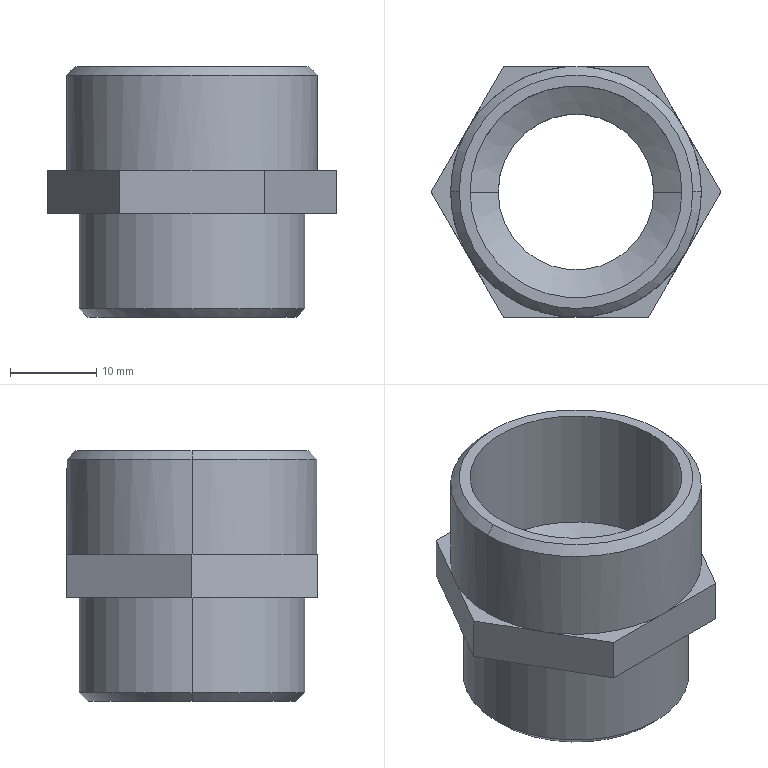Part | SolidWorks | features ICE 3, Chamfer 1, Extrusion 1, HoleWzd 1 | 1 solid | 29 faces | box 33.486 x 29 x 29 mm | volume 7069 mm3 | plane 15 | cylinder 8 | cone 6 | commonest cylinder face diameters 18 x2 24.5 x2 26.1 x2 29 x2
STEP:
#1=CARTESIAN_POINT('',(13.5,0.,14.5));
#2=VERTEX_POINT('',#1);
#3=CARTESIAN_POINT('',(-13.5,0.,14.5));
#4=VERTEX_POINT('',#3);
#5=CARTESIAN_POINT('',(0.,0.,14.5));
#6=DIRECTION('',(0.,0.,1.));
#7=DIRECTION('',(1.,0.,0.));
#8=AXIS2_PLACEMENT_3D('',#5,#6,#7);
#9=CIRCLE('',#8,13.5);
#10=EDGE_CURVE('',#2,#4,#9,.T.);
#11=ORIENTED_EDGE('',*,*,#10,.F.);
#12=CARTESIAN_POINT('',(14.5,0.,13.5));
#13=VERTEX_POINT('',#12);
#14=CARTESIAN_POINT('',(13.5,0.,14.5));
#15=DIRECTION('',(0.7071,0.,-0.7071));
#16=VECTOR('',#15,1000.);
#17=LINE('',#14,#16);
#18=EDGE_CURVE('',#2,#13,#17,.T.);
#19=ORIENTED_EDGE('',*,*,#18,.T.);
#20=CARTESIAN_POINT('',(-14.5,0.,13.5));
#21=VERTEX_POINT('',#20);
#22=CARTESIAN_POINT('',(0.,0.,13.5));
#23=DIRECTION('',(0.,0.,-1.));
#24=DIRECTION('',(1.,0.,0.));
#25=AXIS2_PLACEMENT_3D('',#22,#23,#24);
#26=CIRCLE('',#25,14.5);
#27=EDGE_CURVE('',#21,#13,#26,.T.);
#28=ORIENTED_EDGE('',*,*,#27,.F.);
#29=CARTESIAN_POINT('',(-13.5,0.,14.5));
#30=DIRECTION('',(-0.7071,0.,-0.7071));
#31=VECTOR('',#30,1000.);
#32=LINE('',#29,#31);
#33=EDGE_CURVE('',#4,#21,#32,.T.);
#34=ORIENTED_EDGE('',*,*,#33,.F.);
#35=EDGE_LOOP('',(#11,#19,#28,#34));
#36=FACE_OUTER_BOUND('',#35,.T.);
#37=CARTESIAN_POINT('',(0.,0.,14.5));
#38=DIRECTION('',(0.,0.,-1.));
#39=DIRECTION('',(-1.,0.,0.));
#40=AXIS2_PLACEMENT_3D('',#37,#38,#39);
#41=CONICAL_SURFACE('',#40,13.5,0.7854);
#42=ADVANCED_FACE('',(#36),#41,.T.);
#43=CARTESIAN_POINT('',(-12.05,0.,-14.5));
#44=VERTEX_POINT('',#43);
#45=CARTESIAN_POINT('',(12.05,0.,-14.5));
#46=VERTEX_POINT('',#45);
#47=CARTESIAN_POINT('',(0.,0.,-14.5));
#48=DIRECTION('',(0.,0.,-1.));
#49=DIRECTION('',(-1.,0.,0.));
#50=AXIS2_PLACEMENT_3D('',#47,#48,#49);
#51=CIRCLE('',#50,12.05);
#52=EDGE_CURVE('',#44,#46,#51,.T.);
#53=ORIENTED_EDGE('',*,*,#52,.F.);
#54=CARTESIAN_POINT('',(-13.05,0.,-13.5));
#55=VERTEX_POINT('',#54);
#56=CARTESIAN_POINT('',(-12.05,0.,-14.5));
#57=DIRECTION('',(-0.7071,0.,0.7071));
#58=VECTOR('',#57,1000.);
#59=LINE('',#56,#58);
#60=EDGE_CURVE('',#44,#55,#59,.T.);
#61=ORIENTED_EDGE('',*,*,#60,.T.);
#62=CARTESIAN_POINT('',(13.05,0.,-13.5));
#63=VERTEX_POINT('',#62);
#64=CARTESIAN_POINT('',(0.,0.,-13.5));
#65=DIRECTION('',(0.,0.,1.));
#66=DIRECTION('',(-1.,0.,0.));
#67=AXIS2_PLACEMENT_3D('',#64,#65,#66);
#68=CIRCLE('',#67,13.05);
#69=EDGE_CURVE('',#63,#55,#68,.T.);
#70=ORIENTED_EDGE('',*,*,#69,.F.);
#71=CARTESIAN_POINT('',(12.05,0.,-14.5));
#72=DIRECTION('',(0.7071,0.,0.7071));
#73=VECTOR('',#72,1000.);
#74=LINE('',#71,#73);
#75=EDGE_CURVE('',#46,#63,#74,.T.);
#76=ORIENTED_EDGE('',*,*,#75,.F.);
#77=EDGE_LOOP('',(#53,#61,#70,#76));
#78=FACE_OUTER_BOUND('',#77,.T.);
#79=CARTESIAN_POINT('',(0.,0.,-14.5));
#80=DIRECTION('',(0.,0.,1.));
#81=DIRECTION('',(1.,0.,0.));
#82=AXIS2_PLACEMENT_3D('',#79,#80,#81);
#83=CONICAL_SURFACE('',#82,12.05,0.7854);
#84=ADVANCED_FACE('',(#78),#83,.T.);
#85=CARTESIAN_POINT('',(-12.25,0.,-0.5));
#86=VERTEX_POINT('',#85);
#87=CARTESIAN_POINT('',(12.25,0.,-0.5));
#88=VERTEX_POINT('',#87);
#89=CARTESIAN_POINT('',(0.,0.,-0.5));
#90=DIRECTION('',(0.,0.,1.));
#91=DIRECTION('',(1.,0.,0.));
#92=AXIS2_PLACEMENT_3D('',#89,#90,#91);
#93=CIRCLE('',#92,12.25);
#94=EDGE_CURVE('',#86,#88,#93,.T.);
#95=ORIENTED_EDGE('',*,*,#94,.F.);
#96=CARTESIAN_POINT('',(-12.25,0.,14.5));
#97=VERTEX_POINT('',#96);
#98=CARTESIAN_POINT('',(-12.25,0.,14.5));
#99=DIRECTION('',(0.,0.,1.));
#100=VECTOR('',#99,1000.);
#101=LINE('',#98,#100);
#102=EDGE_CURVE('',#86,#97,#101,.T.);
#103=ORIENTED_EDGE('',*,*,#102,.T.);
#104=CARTESIAN_POINT('',(12.25,0.,14.5));
#105=VERTEX_POINT('',#104);
#106=CARTESIAN_POINT('',(0.,0.,14.5));
#107=DIRECTION('',(0.,0.,1.));
#108=DIRECTION('',(1.,0.,0.));
#109=AXIS2_PLACEMENT_3D('',#106,#107,#108);
#110=CIRCLE('',#109,12.25);
#111=EDGE_CURVE('',#97,#105,#110,.T.);
#112=ORIENTED_EDGE('',*,*,#111,.T.);
#113=CARTESIAN_POINT('',(12.25,0.,14.5));
#114=DIRECTION('',(0.,0.,1.));
#115=VECTOR('',#114,1000.);
#116=LINE('',#113,#115);
#117=EDGE_CURVE('',#88,#105,#116,.T.);
#118=ORIENTED_EDGE('',*,*,#117,.F.);
#119=EDGE_LOOP('',(#95,#103,#112,#118));
#120=FACE_OUTER_BOUND('',#119,.T.);
#121=CARTESIAN_POINT('',(0.,0.,14.5));
#122=DIRECTION('',(0.,0.,1.));
#123=DIRECTION('',(1.,0.,0.));
#124=AXIS2_PLACEMENT_3D('',#121,#122,#123);
#125=CYLINDRICAL_SURFACE('',#124,12.25);
#126=ADVANCED_FACE('',(#120),#125,.F.);
#127=CARTESIAN_POINT('',(-9.,0.,-2.453));
#128=VERTEX_POINT('',#127);
#129=CARTESIAN_POINT('',(9.,0.,-2.453));
#130=VERTEX_POINT('',#129);
#131=CARTESIAN_POINT('',(0.,0.,-2.453));
#132=DIRECTION('',(0.,0.,1.));
#133=DIRECTION('',(1.,0.,0.));
#134=AXIS2_PLACEMENT_3D('',#131,#132,#133);
#135=CIRCLE('',#134,9.);
#136=EDGE_CURVE('',#128,#130,#135,.T.);
#137=ORIENTED_EDGE('',*,*,#136,.F.);
#138=CARTESIAN_POINT('',(-12.25,0.,-0.5));
#139=DIRECTION('',(-0.8572,0.,0.515));
#140=VECTOR('',#139,1000.);
#141=LINE('',#138,#140);
#142=EDGE_CURVE('',#128,#86,#141,.T.);
#143=ORIENTED_EDGE('',*,*,#142,.T.);
#144=ORIENTED_EDGE('',*,*,#94,.T.);
#145=CARTESIAN_POINT('',(12.25,0.,-0.5));
#146=DIRECTION('',(0.8572,0.,0.515));
#147=VECTOR('',#146,1000.);
#148=LINE('',#145,#147);
#149=EDGE_CURVE('',#130,#88,#148,.T.);
#150=ORIENTED_EDGE('',*,*,#149,.F.);
#151=EDGE_LOOP('',(#137,#143,#144,#150));
#152=FACE_OUTER_BOUND('',#151,.T.);
#153=CARTESIAN_POINT('',(0.,0.,-0.5));
#154=DIRECTION('',(0.,0.,1.));
#155=DIRECTION('',(1.,0.,0.));
#156=AXIS2_PLACEMENT_3D('',#153,#154,#155);
#157=CONICAL_SURFACE('',#156,12.25,1.03);
#158=ADVANCED_FACE('',(#152),#157,.F.);
#159=ORIENTED_EDGE('',*,*,#27,.T.);
#160=CARTESIAN_POINT('',(14.5,0.,2.5));
#161=VERTEX_POINT('',#160);
#162=CARTESIAN_POINT('',(14.5,0.,14.5));
#163=DIRECTION('',(0.,0.,-1.));
#164=VECTOR('',#163,1000.);
#165=LINE('',#162,#164);
#166=EDGE_CURVE('',#13,#161,#165,.T.);
#167=ORIENTED_EDGE('',*,*,#166,.T.);
#168=CARTESIAN_POINT('',(12.557,7.25,2.5));
#169=VERTEX_POINT('',#168);
#170=CARTESIAN_POINT('',(0.,0.,2.5));
#171=DIRECTION('',(0.,0.,1.));
#172=DIRECTION('',(1.,0.,0.));
#173=AXIS2_PLACEMENT_3D('',#170,#171,#172);
#174=CIRCLE('',#173,14.5);
#175=EDGE_CURVE('',#161,#169,#174,.T.);
#176=ORIENTED_EDGE('',*,*,#175,.T.);
#177=CARTESIAN_POINT('',(0.,14.5,2.5));
#178=VERTEX_POINT('',#177);
#179=CARTESIAN_POINT('',(0.,0.,2.5));
#180=DIRECTION('',(0.,0.,1.));
#181=DIRECTION('',(1.,0.,0.));
#182=AXIS2_PLACEMENT_3D('',#179,#180,#181);
#183=CIRCLE('',#182,14.5);
#184=EDGE_CURVE('',#169,#178,#183,.T.);
#185=ORIENTED_EDGE('',*,*,#184,.T.);
#186=CARTESIAN_POINT('',(-12.557,7.25,2.5));
#187=VERTEX_POINT('',#186);
#188=CARTESIAN_POINT('',(0.,0.,2.5));
#189=DIRECTION('',(0.,0.,1.));
#190=DIRECTION('',(1.,0.,0.));
#191=AXIS2_PLACEMENT_3D('',#188,#189,#190);
#192=CIRCLE('',#191,14.5);
#193=EDGE_CURVE('',#178,#187,#192,.T.);
#194=ORIENTED_EDGE('',*,*,#193,.T.);
#195=CARTESIAN_POINT('',(-14.5,0.,2.5));
#196=VERTEX_POINT('',#195);
#197=CARTESIAN_POINT('',(0.,0.,2.5));
#198=DIRECTION('',(0.,0.,1.));
#199=DIRECTION('',(1.,0.,0.));
#200=AXIS2_PLACEMENT_3D('',#197,#198,#199);
#201=CIRCLE('',#200,14.5);
#202=EDGE_CURVE('',#187,#196,#201,.T.);
#203=ORIENTED_EDGE('',*,*,#202,.T.);
#204=CARTESIAN_POINT('',(-14.5,0.,14.5));
#205=DIRECTION('',(0.,0.,-1.));
#206=VECTOR('',#205,1000.);
#207=LINE('',#204,#206);
#208=EDGE_CURVE('',#21,#196,#207,.T.);
#209=ORIENTED_EDGE('',*,*,#208,.F.);
#210=EDGE_LOOP('',(#159,#167,#176,#185,#194,#203,#209));
#211=FACE_OUTER_BOUND('',#210,.T.);
#212=CARTESIAN_POINT('',(0.,0.,14.5));
#213=DIRECTION('',(0.,0.,-1.));
#214=DIRECTION('',(-1.,0.,0.));
#215=AXIS2_PLACEMENT_3D('',#212,#213,#214);
#216=CYLINDRICAL_SURFACE('',#215,14.5);
#217=ADVANCED_FACE('',(#211),#216,.T.);
#218=ORIENTED_EDGE('',*,*,#136,.T.);
#219=CARTESIAN_POINT('',(9.,0.,-14.5));
#220=VERTEX_POINT('',#219);
#221=CARTESIAN_POINT('',(9.,0.,2.501));
#222=DIRECTION('',(0.,0.,-1.));
#223=VECTOR('',#222,1000.);
#224=LINE('',#221,#223);
#225=EDGE_CURVE('',#130,#220,#224,.T.);
#226=ORIENTED_EDGE('',*,*,#225,.T.);
#227=CARTESIAN_POINT('',(-9.,0.,-14.5));
#228=VERTEX_POINT('',#227);
#229=CARTESIAN_POINT('',(0.,0.,-14.5));
#230=DIRECTION('',(0.,0.,-1.));
#231=DIRECTION('',(-1.,0.,0.));
#232=AXIS2_PLACEMENT_3D('',#229,#230,#231);
#233=CIRCLE('',#232,9.);
#234=EDGE_CURVE('',#220,#228,#233,.T.);
#235=ORIENTED_EDGE('',*,*,#234,.T.);
#236=CARTESIAN_POINT('',(-9.,0.,2.501));
#237=DIRECTION('',(0.,0.,-1.));
#238=VECTOR('',#237,1000.);
#239=LINE('',#236,#238);
#240=EDGE_CURVE('',#128,#228,#239,.T.);
#241=ORIENTED_EDGE('',*,*,#240,.F.);
#242=EDGE_LOOP('',(#218,#226,#235,#241));
#243=FACE_OUTER_BOUND('',#242,.T.);
#244=CARTESIAN_POINT('',(0.,0.,2.501));
#245=DIRECTION('',(0.,0.,-1.));
#246=DIRECTION('',(-1.,0.,0.));
#247=AXIS2_PLACEMENT_3D('',#244,#245,#246);
#248=CYLINDRICAL_SURFACE('',#247,9.);
#249=ADVANCED_FACE('',(#243),#248,.F.);
#250=ORIENTED_EDGE('',*,*,#69,.T.);
#251=CARTESIAN_POINT('',(-13.05,0.,-2.5));
#252=VERTEX_POINT('',#251);
#253=CARTESIAN_POINT('',(-13.05,0.,-14.5));
#254=DIRECTION('',(0.,0.,1.));
#255=VECTOR('',#254,1000.);
#256=LINE('',#253,#255);
#257=EDGE_CURVE('',#55,#252,#256,.T.);
#258=ORIENTED_EDGE('',*,*,#257,.T.);
#259=CARTESIAN_POINT('',(13.05,0.,-2.5));
#260=VERTEX_POINT('',#259);
#261=CARTESIAN_POINT('',(0.,0.,-2.5));
#262=DIRECTION('',(0.,0.,-1.));
#263=DIRECTION('',(-1.,0.,0.));
#264=AXIS2_PLACEMENT_3D('',#261,#262,#263);
#265=CIRCLE('',#264,13.05);
#266=EDGE_CURVE('',#252,#260,#265,.T.);
#267=ORIENTED_EDGE('',*,*,#266,.T.);
#268=CARTESIAN_POINT('',(13.05,0.,-14.5));
#269=DIRECTION('',(0.,0.,1.));
#270=VECTOR('',#269,1000.);
#271=LINE('',#268,#270);
#272=EDGE_CURVE('',#63,#260,#271,.T.);
#273=ORIENTED_EDGE('',*,*,#272,.F.);
#274=EDGE_LOOP('',(#250,#258,#267,#273));
#275=FACE_OUTER_BOUND('',#274,.T.);
#276=CARTESIAN_POINT('',(0.,0.,-14.5));
#277=DIRECTION('',(0.,0.,1.));
#278=DIRECTION('',(1.,0.,0.));
#279=AXIS2_PLACEMENT_3D('',#276,#277,#278);
#280=CYLINDRICAL_SURFACE('',#279,13.05);
#281=ADVANCED_FACE('',(#275),#280,.T.);
#282=ORIENTED_EDGE('',*,*,#184,.F.);
#283=CARTESIAN_POINT('',(8.372,14.5,2.5));
#284=VERTEX_POINT('',#283);
#285=CARTESIAN_POINT('',(16.743,0.,2.5));
#286=DIRECTION('',(-0.5,0.866,0.));
#287=VECTOR('',#286,1000.);
#288=LINE('',#285,#287);
#289=EDGE_CURVE('',#169,#284,#288,.T.);
#290=ORIENTED_EDGE('',*,*,#289,.T.);
#291=CARTESIAN_POINT('',(8.372,14.5,2.5));
#292=DIRECTION('',(-1.,0.,0.));
#293=VECTOR('',#292,1000.);
#294=LINE('',#291,#293);
#295=EDGE_CURVE('',#284,#178,#294,.T.);
#296=ORIENTED_EDGE('',*,*,#295,.T.);
#297=EDGE_LOOP('',(#282,#290,#296));
#298=FACE_OUTER_BOUND('',#297,.T.);
#299=CARTESIAN_POINT('',(0.,0.,2.5));
#300=DIRECTION('',(0.,0.,1.));
#301=DIRECTION('',(1.,0.,0.));
#302=AXIS2_PLACEMENT_3D('',#299,#300,#301);
#303=PLANE('',#302);
#304=ADVANCED_FACE('',(#298),#303,.T.);
#305=ORIENTED_EDGE('',*,*,#193,.F.);
#306=CARTESIAN_POINT('',(-8.372,14.5,2.5));
#307=VERTEX_POINT('',#306);
#308=CARTESIAN_POINT('',(8.372,14.5,2.5));
#309=DIRECTION('',(-1.,0.,0.));
#310=VECTOR('',#309,1000.);
#311=LINE('',#308,#310);
#312=EDGE_CURVE('',#178,#307,#311,.T.);
#313=ORIENTED_EDGE('',*,*,#312,.T.);
#314=CARTESIAN_POINT('',(-8.372,14.5,2.5));
#315=DIRECTION('',(-0.5,-0.866,0.));
#316=VECTOR('',#315,1000.);
#317=LINE('',#314,#316);
#318=EDGE_CURVE('',#307,#187,#317,.T.);
#319=ORIENTED_EDGE('',*,*,#318,.T.);
#320=EDGE_LOOP('',(#305,#313,#319));
#321=FACE_OUTER_BOUND('',#320,.T.);
#322=CARTESIAN_POINT('',(0.,0.,2.5));
#323=DIRECTION('',(0.,0.,1.));
#324=DIRECTION('',(1.,0.,0.));
#325=AXIS2_PLACEMENT_3D('',#322,#323,#324);
#326=PLANE('',#325);
#327=ADVANCED_FACE('',(#321),#326,.T.);
#328=ORIENTED_EDGE('',*,*,#202,.F.);
#329=CARTESIAN_POINT('',(-16.743,0.,2.5));
#330=VERTEX_POINT('',#329);
#331=CARTESIAN_POINT('',(-8.372,14.5,2.5));
#332=DIRECTION('',(-0.5,-0.866,0.));
#333=VECTOR('',#332,1000.);
#334=LINE('',#331,#333);
#335=EDGE_CURVE('',#187,#330,#334,.T.);
#336=ORIENTED_EDGE('',*,*,#335,.T.);
#337=CARTESIAN_POINT('',(-12.557,-7.25,2.5));
#338=VERTEX_POINT('',#337);
#339=CARTESIAN_POINT('',(-16.743,0.,2.5));
#340=DIRECTION('',(0.5,-0.866,0.));
#341=VECTOR('',#340,1000.);
#342=LINE('',#339,#341);
#343=EDGE_CURVE('',#330,#338,#342,.T.);
#344=ORIENTED_EDGE('',*,*,#343,.T.);
#345=CARTESIAN_POINT('',(0.,0.,2.5));
#346=DIRECTION('',(0.,0.,1.));
#347=DIRECTION('',(1.,0.,0.));
#348=AXIS2_PLACEMENT_3D('',#345,#346,#347);
#349=CIRCLE('',#348,14.5);
#350=EDGE_CURVE('',#196,#338,#349,.T.);
#351=ORIENTED_EDGE('',*,*,#350,.F.);
#352=EDGE_LOOP('',(#328,#336,#344,#351));
#353=FACE_OUTER_BOUND('',#352,.T.);
#354=CARTESIAN_POINT('',(0.,0.,2.5));
#355=DIRECTION('',(0.,0.,1.));
#356=DIRECTION('',(1.,0.,0.));
#357=AXIS2_PLACEMENT_3D('',#354,#355,#356);
#358=PLANE('',#357);
#359=ADVANCED_FACE('',(#353),#358,.T.);
#360=CARTESIAN_POINT('',(0.,-14.5,2.5));
#361=VERTEX_POINT('',#360);
#362=CARTESIAN_POINT('',(0.,0.,2.5));
#363=DIRECTION('',(0.,0.,1.));
#364=DIRECTION('',(1.,0.,0.));
#365=AXIS2_PLACEMENT_3D('',#362,#363,#364);
#366=CIRCLE('',#365,14.5);
#367=EDGE_CURVE('',#338,#361,#366,.T.);
#368=ORIENTED_EDGE('',*,*,#367,.F.);
#369=CARTESIAN_POINT('',(-8.372,-14.5,2.5));
#370=VERTEX_POINT('',#369);
#371=CARTESIAN_POINT('',(-16.743,0.,2.5));
#372=DIRECTION('',(0.5,-0.866,0.));
#373=VECTOR('',#372,1000.);
#374=LINE('',#371,#373);
#375=EDGE_CURVE('',#338,#370,#374,.T.);
#376=ORIENTED_EDGE('',*,*,#375,.T.);
#377=CARTESIAN_POINT('',(-8.372,-14.5,2.5));
#378=DIRECTION('',(1.,0.,0.));
#379=VECTOR('',#378,1000.);
#380=LINE('',#377,#379);
#381=EDGE_CURVE('',#370,#361,#380,.T.);
#382=ORIENTED_EDGE('',*,*,#381,.T.);
#383=EDGE_LOOP('',(#368,#376,#382));
#384=FACE_OUTER_BOUND('',#383,.T.);
#385=CARTESIAN_POINT('',(0.,0.,2.5));
#386=DIRECTION('',(0.,0.,1.));
#387=DIRECTION('',(1.,0.,0.));
#388=AXIS2_PLACEMENT_3D('',#385,#386,#387);
#389=PLANE('',#388);
#390=ADVANCED_FACE('',(#384),#389,.T.);
#391=CARTESIAN_POINT('',(12.557,-7.25,2.5));
#392=VERTEX_POINT('',#391);
#393=CARTESIAN_POINT('',(0.,0.,2.5));
#394=DIRECTION('',(0.,0.,1.));
#395=DIRECTION('',(1.,0.,0.));
#396=AXIS2_PLACEMENT_3D('',#393,#394,#395);
#397=CIRCLE('',#396,14.5);
#398=EDGE_CURVE('',#361,#392,#397,.T.);
#399=ORIENTED_EDGE('',*,*,#398,.F.);
#400=CARTESIAN_POINT('',(8.372,-14.5,2.5));
#401=VERTEX_POINT('',#400);
#402=CARTESIAN_POINT('',(-8.372,-14.5,2.5));
#403=DIRECTION('',(1.,0.,0.));
#404=VECTOR('',#403,1000.);
#405=LINE('',#402,#404);
#406=EDGE_CURVE('',#361,#401,#405,.T.);
#407=ORIENTED_EDGE('',*,*,#406,.T.);
#408=CARTESIAN_POINT('',(8.372,-14.5,2.5));
#409=DIRECTION('',(0.5,0.866,0.));
#410=VECTOR('',#409,1000.);
#411=LINE('',#408,#410);
#412=EDGE_CURVE('',#401,#392,#411,.T.);
#413=ORIENTED_EDGE('',*,*,#412,.T.);
#414=EDGE_LOOP('',(#399,#407,#413));
#415=FACE_OUTER_BOUND('',#414,.T.);
#416=CARTESIAN_POINT('',(0.,0.,2.5));
#417=DIRECTION('',(0.,0.,1.));
#418=DIRECTION('',(1.,0.,0.));
#419=AXIS2_PLACEMENT_3D('',#416,#417,#418);
#420=PLANE('',#419);
#421=ADVANCED_FACE('',(#415),#420,.T.);
#422=CARTESIAN_POINT('',(8.372,-14.5,-2.5));
#423=VERTEX_POINT('',#422);
#424=CARTESIAN_POINT('',(16.743,0.,-2.5));
#425=VERTEX_POINT('',#424);
#426=CARTESIAN_POINT('',(8.372,-14.5,-2.5));
#427=DIRECTION('',(0.5,0.866,0.));
#428=VECTOR('',#427,1000.);
#429=LINE('',#426,#428);
#430=EDGE_CURVE('',#423,#425,#429,.T.);
#431=ORIENTED_EDGE('',*,*,#430,.T.);
#432=CARTESIAN_POINT('',(16.743,0.,2.5));
#433=VERTEX_POINT('',#432);
#434=CARTESIAN_POINT('',(16.743,0.,2.5));
#435=DIRECTION('',(0.,0.,-1.));
#436=VECTOR('',#435,1000.);
#437=LINE('',#434,#436);
#438=EDGE_CURVE('',#433,#425,#437,.T.);
#439=ORIENTED_EDGE('',*,*,#438,.F.);
#440=CARTESIAN_POINT('',(8.372,-14.5,2.5));
#441=DIRECTION('',(0.5,0.866,0.));
#442=VECTOR('',#441,1000.);
#443=LINE('',#440,#442);
#444=EDGE_CURVE('',#392,#433,#443,.T.);
#445=ORIENTED_EDGE('',*,*,#444,.F.);
#446=ORIENTED_EDGE('',*,*,#412,.F.);
#447=CARTESIAN_POINT('',(8.372,-14.5,2.5));
#448=DIRECTION('',(0.,0.,-1.));
#449=VECTOR('',#448,1000.);
#450=LINE('',#447,#449);
#451=EDGE_CURVE('',#401,#423,#450,.T.);
#452=ORIENTED_EDGE('',*,*,#451,.T.);
#453=EDGE_LOOP('',(#431,#439,#445,#446,#452));
#454=FACE_OUTER_BOUND('',#453,.T.);
#455=CARTESIAN_POINT('',(8.372,-14.5,2.5));
#456=DIRECTION('',(-0.866,0.5,0.));
#457=DIRECTION('',(-0.5,-0.866,0.));
#458=AXIS2_PLACEMENT_3D('',#455,#456,#457);
#459=PLANE('',#458);
#460=ADVANCED_FACE('',(#454),#459,.F.);
#461=CARTESIAN_POINT('',(8.372,14.5,-2.5));
#462=VERTEX_POINT('',#461);
#463=CARTESIAN_POINT('',(16.743,0.,-2.5));
#464=DIRECTION('',(-0.5,0.866,0.));
#465=VECTOR('',#464,1000.);
#466=LINE('',#463,#465);
#467=EDGE_CURVE('',#425,#462,#466,.T.);
#468=ORIENTED_EDGE('',*,*,#467,.T.);
#469=CARTESIAN_POINT('',(8.372,14.5,2.5));
#470=DIRECTION('',(0.,0.,-1.));
#471=VECTOR('',#470,1000.);
#472=LINE('',#469,#471);
#473=EDGE_CURVE('',#284,#462,#472,.T.);
#474=ORIENTED_EDGE('',*,*,#473,.F.);
#475=ORIENTED_EDGE('',*,*,#289,.F.);
#476=CARTESIAN_POINT('',(16.743,0.,2.5));
#477=DIRECTION('',(-0.5,0.866,0.));
#478=VECTOR('',#477,1000.);
#479=LINE('',#476,#478);
#480=EDGE_CURVE('',#433,#169,#479,.T.);
#481=ORIENTED_EDGE('',*,*,#480,.F.);
#482=ORIENTED_EDGE('',*,*,#438,.T.);
#483=EDGE_LOOP('',(#468,#474,#475,#481,#482));
#484=FACE_OUTER_BOUND('',#483,.T.);
#485=CARTESIAN_POINT('',(16.743,0.,2.5));
#486=DIRECTION('',(-0.866,-0.5,0.));
#487=DIRECTION('',(0.5,-0.866,0.));
#488=AXIS2_PLACEMENT_3D('',#485,#486,#487);
#489=PLANE('',#488);
#490=ADVANCED_FACE('',(#484),#489,.F.);
#491=CARTESIAN_POINT('',(-8.372,14.5,-2.5));
#492=VERTEX_POINT('',#491);
#493=CARTESIAN_POINT('',(8.372,14.5,-2.5));
#494=DIRECTION('',(-1.,0.,0.));
#495=VECTOR('',#494,1000.);
#496=LINE('',#493,#495);
#497=EDGE_CURVE('',#462,#492,#496,.T.);
#498=ORIENTED_EDGE('',*,*,#497,.T.);
#499=CARTESIAN_POINT('',(-8.372,14.5,2.5));
#500=DIRECTION('',(0.,0.,-1.));
#501=VECTOR('',#500,1000.);
#502=LINE('',#499,#501);
#503=EDGE_CURVE('',#307,#492,#502,.T.);
#504=ORIENTED_EDGE('',*,*,#503,.F.);
#505=ORIENTED_EDGE('',*,*,#312,.F.);
#506=ORIENTED_EDGE('',*,*,#295,.F.);
#507=ORIENTED_EDGE('',*,*,#473,.T.);
#508=EDGE_LOOP('',(#498,#504,#505,#506,#507));
#509=FACE_OUTER_BOUND('',#508,.T.);
#510=CARTESIAN_POINT('',(8.372,14.5,2.5));
#511=DIRECTION('',(0.,-1.,0.));
#512=DIRECTION('',(0.,0.,-1.));
#513=AXIS2_PLACEMENT_3D('',#510,#511,#512);
#514=PLANE('',#513);
#515=ADVANCED_FACE('',(#509),#514,.F.);
#516=CARTESIAN_POINT('',(-16.743,0.,-2.5));
#517=VERTEX_POINT('',#516);
#518=CARTESIAN_POINT('',(-8.372,14.5,-2.5));
#519=DIRECTION('',(-0.5,-0.866,0.));
#520=VECTOR('',#519,1000.);
#521=LINE('',#518,#520);
#522=EDGE_CURVE('',#492,#517,#521,.T.);
#523=ORIENTED_EDGE('',*,*,#522,.T.);
#524=CARTESIAN_POINT('',(-16.743,0.,2.5));
#525=DIRECTION('',(0.,0.,-1.));
#526=VECTOR('',#525,1000.);
#527=LINE('',#524,#526);
#528=EDGE_CURVE('',#330,#517,#527,.T.);
#529=ORIENTED_EDGE('',*,*,#528,.F.);
#530=ORIENTED_EDGE('',*,*,#335,.F.);
#531=ORIENTED_EDGE('',*,*,#318,.F.);
#532=ORIENTED_EDGE('',*,*,#503,.T.);
#533=EDGE_LOOP('',(#523,#529,#530,#531,#532));
#534=FACE_OUTER_BOUND('',#533,.T.);
#535=CARTESIAN_POINT('',(-8.372,14.5,2.5));
#536=DIRECTION('',(0.866,-0.5,0.));
#537=DIRECTION('',(0.5,0.866,0.));
#538=AXIS2_PLACEMENT_3D('',#535,#536,#537);
#539=PLANE('',#538);
#540=ADVANCED_FACE('',(#534),#539,.F.);
#541=CARTESIAN_POINT('',(-8.372,-14.5,-2.5));
#542=VERTEX_POINT('',#541);
#543=CARTESIAN_POINT('',(-16.743,0.,-2.5));
#544=DIRECTION('',(0.5,-0.866,0.));
#545=VECTOR('',#544,1000.);
#546=LINE('',#543,#545);
#547=EDGE_CURVE('',#517,#542,#546,.T.);
#548=ORIENTED_EDGE('',*,*,#547,.T.);
#549=CARTESIAN_POINT('',(-8.372,-14.5,2.5));
#550=DIRECTION('',(0.,0.,-1.));
#551=VECTOR('',#550,1000.);
#552=LINE('',#549,#551);
#553=EDGE_CURVE('',#370,#542,#552,.T.);
#554=ORIENTED_EDGE('',*,*,#553,.F.);
#555=ORIENTED_EDGE('',*,*,#375,.F.);
#556=ORIENTED_EDGE('',*,*,#343,.F.);
#557=ORIENTED_EDGE('',*,*,#528,.T.);
#558=EDGE_LOOP('',(#548,#554,#555,#556,#557));
#559=FACE_OUTER_BOUND('',#558,.T.);
#560=CARTESIAN_POINT('',(-16.743,0.,2.5));
#561=DIRECTION('',(0.866,0.5,0.));
#562=DIRECTION('',(-0.5,0.866,0.));
#563=AXIS2_PLACEMENT_3D('',#560,#561,#562);
#564=PLANE('',#563);
#565=ADVANCED_FACE('',(#559),#564,.F.);
#566=CARTESIAN_POINT('',(-8.372,-14.5,-2.5));
#567=DIRECTION('',(1.,0.,0.));
#568=VECTOR('',#567,1000.);
#569=LINE('',#566,#568);
#570=EDGE_CURVE('',#542,#423,#569,.T.);
#571=ORIENTED_EDGE('',*,*,#570,.T.);
#572=ORIENTED_EDGE('',*,*,#451,.F.);
#573=ORIENTED_EDGE('',*,*,#406,.F.);
#574=ORIENTED_EDGE('',*,*,#381,.F.);
#575=ORIENTED_EDGE('',*,*,#553,.T.);
#576=EDGE_LOOP('',(#571,#572,#573,#574,#575));
#577=FACE_OUTER_BOUND('',#576,.T.);
#578=CARTESIAN_POINT('',(-8.372,-14.5,2.5));
#579=DIRECTION('',(0.,1.,0.));
#580=DIRECTION('',(-1.,0.,0.));
#581=AXIS2_PLACEMENT_3D('',#578,#579,#580);
#582=PLANE('',#581);
#583=ADVANCED_FACE('',(#577),#582,.F.);
#584=CARTESIAN_POINT('',(0.,0.,2.5));
#585=DIRECTION('',(0.,0.,1.));
#586=DIRECTION('',(1.,0.,0.));
#587=AXIS2_PLACEMENT_3D('',#584,#585,#586);
#588=CIRCLE('',#587,14.5);
#589=EDGE_CURVE('',#392,#161,#588,.T.);
#590=ORIENTED_EDGE('',*,*,#589,.F.);
#591=ORIENTED_EDGE('',*,*,#444,.T.);
#592=ORIENTED_EDGE('',*,*,#480,.T.);
#593=ORIENTED_EDGE('',*,*,#175,.F.);
#594=EDGE_LOOP('',(#590,#591,#592,#593));
#595=FACE_OUTER_BOUND('',#594,.T.);
#596=CARTESIAN_POINT('',(0.,0.,2.5));
#597=DIRECTION('',(0.,0.,1.));
#598=DIRECTION('',(1.,0.,0.));
#599=AXIS2_PLACEMENT_3D('',#596,#597,#598);
#600=PLANE('',#599);
#601=ADVANCED_FACE('',(#595),#600,.T.);
#602=CARTESIAN_POINT('',(0.,0.,-2.5));
#603=DIRECTION('',(0.,0.,-1.));
#604=DIRECTION('',(-1.,0.,0.));
#605=AXIS2_PLACEMENT_3D('',#602,#603,#604);
#606=CIRCLE('',#605,13.05);
#607=EDGE_CURVE('',#260,#252,#606,.T.);
#608=ORIENTED_EDGE('',*,*,#607,.F.);
#609=ORIENTED_EDGE('',*,*,#266,.F.);
#610=EDGE_LOOP('',(#608,#609));
#611=FACE_BOUND('',#610,.T.);
#612=ORIENTED_EDGE('',*,*,#430,.F.);
#613=ORIENTED_EDGE('',*,*,#570,.F.);
#614=ORIENTED_EDGE('',*,*,#547,.F.);
#615=ORIENTED_EDGE('',*,*,#522,.F.);
#616=ORIENTED_EDGE('',*,*,#497,.F.);
#617=ORIENTED_EDGE('',*,*,#467,.F.);
#618=EDGE_LOOP('',(#612,#613,#614,#615,#616,#617));
#619=FACE_OUTER_BOUND('',#618,.T.);
#620=CARTESIAN_POINT('',(0.,0.,-2.5));
#621=DIRECTION('',(0.,0.,1.));
#622=DIRECTION('',(1.,0.,0.));
#623=AXIS2_PLACEMENT_3D('',#620,#621,#622);
#624=PLANE('',#623);
#625=ADVANCED_FACE('',(#611,#619),#624,.F.);
#626=ORIENTED_EDGE('',*,*,#257,.F.);
#627=CARTESIAN_POINT('',(0.,0.,-13.5));
#628=DIRECTION('',(0.,0.,1.));
#629=DIRECTION('',(-1.,0.,0.));
#630=AXIS2_PLACEMENT_3D('',#627,#628,#629);
#631=CIRCLE('',#630,13.05);
#632=EDGE_CURVE('',#55,#63,#631,.T.);
#633=ORIENTED_EDGE('',*,*,#632,.T.);
#634=ORIENTED_EDGE('',*,*,#272,.T.);
#635=ORIENTED_EDGE('',*,*,#607,.T.);
#636=EDGE_LOOP('',(#626,#633,#634,#635));
#637=FACE_OUTER_BOUND('',#636,.T.);
#638=CARTESIAN_POINT('',(0.,0.,-14.5));
#639=DIRECTION('',(0.,0.,1.));
#640=DIRECTION('',(1.,0.,0.));
#641=AXIS2_PLACEMENT_3D('',#638,#639,#640);
#642=CYLINDRICAL_SURFACE('',#641,13.05);
#643=ADVANCED_FACE('',(#637),#642,.T.);
#644=CARTESIAN_POINT('',(0.,0.,-14.5));
#645=DIRECTION('',(0.,0.,-1.));
#646=DIRECTION('',(-1.,0.,0.));
#647=AXIS2_PLACEMENT_3D('',#644,#645,#646);
#648=CIRCLE('',#647,12.05);
#649=EDGE_CURVE('',#46,#44,#648,.T.);
#650=ORIENTED_EDGE('',*,*,#649,.T.);
#651=ORIENTED_EDGE('',*,*,#52,.T.);
#652=EDGE_LOOP('',(#650,#651));
#653=FACE_OUTER_BOUND('',#652,.T.);
#654=CARTESIAN_POINT('',(0.,0.,-14.5));
#655=DIRECTION('',(0.,0.,-1.));
#656=DIRECTION('',(-1.,0.,0.));
#657=AXIS2_PLACEMENT_3D('',#654,#655,#656);
#658=CIRCLE('',#657,9.);
#659=EDGE_CURVE('',#228,#220,#658,.T.);
#660=ORIENTED_EDGE('',*,*,#659,.F.);
#661=ORIENTED_EDGE('',*,*,#234,.F.);
#662=EDGE_LOOP('',(#660,#661));
#663=FACE_BOUND('',#662,.T.);
#664=CARTESIAN_POINT('',(0.,0.,-14.5));
#665=DIRECTION('',(0.,0.,-1.));
#666=DIRECTION('',(-1.,0.,0.));
#667=AXIS2_PLACEMENT_3D('',#664,#665,#666);
#668=PLANE('',#667);
#669=ADVANCED_FACE('',(#653,#663),#668,.T.);
#670=ORIENTED_EDGE('',*,*,#225,.F.);
#671=CARTESIAN_POINT('',(0.,0.,-2.453));
#672=DIRECTION('',(0.,0.,1.));
#673=DIRECTION('',(1.,0.,0.));
#674=AXIS2_PLACEMENT_3D('',#671,#672,#673);
#675=CIRCLE('',#674,9.);
#676=EDGE_CURVE('',#130,#128,#675,.T.);
#677=ORIENTED_EDGE('',*,*,#676,.T.);
#678=ORIENTED_EDGE('',*,*,#240,.T.);
#679=ORIENTED_EDGE('',*,*,#659,.T.);
#680=EDGE_LOOP('',(#670,#677,#678,#679));
#681=FACE_OUTER_BOUND('',#680,.T.);
#682=CARTESIAN_POINT('',(0.,0.,2.501));
#683=DIRECTION('',(0.,0.,-1.));
#684=DIRECTION('',(-1.,0.,0.));
#685=AXIS2_PLACEMENT_3D('',#682,#683,#684);
#686=CYLINDRICAL_SURFACE('',#685,9.);
#687=ADVANCED_FACE('',(#681),#686,.F.);
#688=CARTESIAN_POINT('',(0.,0.,14.5));
#689=DIRECTION('',(0.,0.,1.));
#690=DIRECTION('',(1.,0.,0.));
#691=AXIS2_PLACEMENT_3D('',#688,#689,#690);
#692=CIRCLE('',#691,13.5);
#693=EDGE_CURVE('',#4,#2,#692,.T.);
#694=ORIENTED_EDGE('',*,*,#693,.T.);
#695=ORIENTED_EDGE('',*,*,#10,.T.);
#696=EDGE_LOOP('',(#694,#695));
#697=FACE_OUTER_BOUND('',#696,.T.);
#698=CARTESIAN_POINT('',(0.,0.,14.5));
#699=DIRECTION('',(0.,0.,1.));
#700=DIRECTION('',(1.,0.,0.));
#701=AXIS2_PLACEMENT_3D('',#698,#699,#700);
#702=CIRCLE('',#701,12.25);
#703=EDGE_CURVE('',#105,#97,#702,.T.);
#704=ORIENTED_EDGE('',*,*,#703,.F.);
#705=ORIENTED_EDGE('',*,*,#111,.F.);
#706=EDGE_LOOP('',(#704,#705));
#707=FACE_BOUND('',#706,.T.);
#708=CARTESIAN_POINT('',(0.,0.,14.5));
#709=DIRECTION('',(0.,0.,1.));
#710=DIRECTION('',(1.,0.,0.));
#711=AXIS2_PLACEMENT_3D('',#708,#709,#710);
#712=PLANE('',#711);
#713=ADVANCED_FACE('',(#697,#707),#712,.T.);
#714=ORIENTED_EDGE('',*,*,#166,.F.);
#715=CARTESIAN_POINT('',(0.,0.,13.5));
#716=DIRECTION('',(0.,0.,-1.));
#717=DIRECTION('',(1.,0.,0.));
#718=AXIS2_PLACEMENT_3D('',#715,#716,#717);
#719=CIRCLE('',#718,14.5);
#720=EDGE_CURVE('',#13,#21,#719,.T.);
#721=ORIENTED_EDGE('',*,*,#720,.T.);
#722=ORIENTED_EDGE('',*,*,#208,.T.);
#723=ORIENTED_EDGE('',*,*,#350,.T.);
#724=ORIENTED_EDGE('',*,*,#367,.T.);
#725=ORIENTED_EDGE('',*,*,#398,.T.);
#726=ORIENTED_EDGE('',*,*,#589,.T.);
#727=EDGE_LOOP('',(#714,#721,#722,#723,#724,#725,#726));
#728=FACE_OUTER_BOUND('',#727,.T.);
#729=CARTESIAN_POINT('',(0.,0.,14.5));
#730=DIRECTION('',(0.,0.,-1.));
#731=DIRECTION('',(-1.,0.,0.));
#732=AXIS2_PLACEMENT_3D('',#729,#730,#731);
#733=CYLINDRICAL_SURFACE('',#732,14.5);
#734=ADVANCED_FACE('',(#728),#733,.T.);
#735=ORIENTED_EDGE('',*,*,#142,.F.);
#736=ORIENTED_EDGE('',*,*,#676,.F.);
#737=ORIENTED_EDGE('',*,*,#149,.T.);
#738=CARTESIAN_POINT('',(0.,0.,-0.5));
#739=DIRECTION('',(0.,0.,1.));
#740=DIRECTION('',(1.,0.,0.));
#741=AXIS2_PLACEMENT_3D('',#738,#739,#740);
#742=CIRCLE('',#741,12.25);
#743=EDGE_CURVE('',#88,#86,#742,.T.);
#744=ORIENTED_EDGE('',*,*,#743,.T.);
#745=EDGE_LOOP('',(#735,#736,#737,#744));
#746=FACE_OUTER_BOUND('',#745,.T.);
#747=CARTESIAN_POINT('',(0.,0.,-0.5));
#748=DIRECTION('',(0.,0.,1.));
#749=DIRECTION('',(1.,0.,0.));
#750=AXIS2_PLACEMENT_3D('',#747,#748,#749);
#751=CONICAL_SURFACE('',#750,12.25,1.03);
#752=ADVANCED_FACE('',(#746),#751,.F.);
#753=ORIENTED_EDGE('',*,*,#102,.F.);
#754=ORIENTED_EDGE('',*,*,#743,.F.);
#755=ORIENTED_EDGE('',*,*,#117,.T.);
#756=ORIENTED_EDGE('',*,*,#703,.T.);
#757=EDGE_LOOP('',(#753,#754,#755,#756));
#758=FACE_OUTER_BOUND('',#757,.T.);
#759=CARTESIAN_POINT('',(0.,0.,14.5));
#760=DIRECTION('',(0.,0.,1.));
#761=DIRECTION('',(1.,0.,0.));
#762=AXIS2_PLACEMENT_3D('',#759,#760,#761);
#763=CYLINDRICAL_SURFACE('',#762,12.25);
#764=ADVANCED_FACE('',(#758),#763,.F.);
#765=ORIENTED_EDGE('',*,*,#60,.F.);
#766=ORIENTED_EDGE('',*,*,#649,.F.);
#767=ORIENTED_EDGE('',*,*,#75,.T.);
#768=ORIENTED_EDGE('',*,*,#632,.F.);
#769=EDGE_LOOP('',(#765,#766,#767,#768));
#770=FACE_OUTER_BOUND('',#769,.T.);
#771=CARTESIAN_POINT('',(0.,0.,-14.5));
#772=DIRECTION('',(0.,0.,1.));
#773=DIRECTION('',(1.,0.,0.));
#774=AXIS2_PLACEMENT_3D('',#771,#772,#773);
#775=CONICAL_SURFACE('',#774,12.05,0.7854);
#776=ADVANCED_FACE('',(#770),#775,.T.);
#777=ORIENTED_EDGE('',*,*,#18,.F.);
#778=ORIENTED_EDGE('',*,*,#693,.F.);
#779=ORIENTED_EDGE('',*,*,#33,.T.);
#780=ORIENTED_EDGE('',*,*,#720,.F.);
#781=EDGE_LOOP('',(#777,#778,#779,#780));
#782=FACE_OUTER_BOUND('',#781,.T.);
#783=CARTESIAN_POINT('',(0.,0.,14.5));
#784=DIRECTION('',(0.,0.,-1.));
#785=DIRECTION('',(-1.,0.,0.));
#786=AXIS2_PLACEMENT_3D('',#783,#784,#785);
#787=CONICAL_SURFACE('',#786,13.5,0.7854);
#788=ADVANCED_FACE('',(#782),#787,.T.);
#789=CLOSED_SHELL('',(#42,#84,#126,#158,#217,#249,#281,#304,#327,#359,#390,#421,#460,#490,#515,#540,#565,#583,#601,#625,#643,#669,#687,#713,#734,#752,#764,#776,#788));
#790=MANIFOLD_SOLID_BREP('',#789);
#791=CARTESIAN_POINT('',(0.,0.,0.));
#792=DIRECTION('',(0.,0.,1.));
#793=DIRECTION('',(1.,0.,0.));
#794=AXIS2_PLACEMENT_3D('',#791,#792,#793);
#795=(LENGTH_UNIT()NAMED_UNIT(*)SI_UNIT(.MILLI.,.METRE.));
#796=UNCERTAINTY_MEASURE_WITH_UNIT(LENGTH_MEASURE(0.00001),#795,'','');
#797=(NAMED_UNIT(*)PLANE_ANGLE_UNIT()SI_UNIT($,.RADIAN.));
#798=(NAMED_UNIT(*)SI_UNIT($,.STERADIAN.)SOLID_ANGLE_UNIT());
#799=(GEOMETRIC_REPRESENTATION_CONTEXT(3)GLOBAL_UNCERTAINTY_ASSIGNED_CONTEXT((#796))GLOBAL_UNIT_ASSIGNED_CONTEXT((#795,#797,#798))REPRESENTATION_CONTEXT('',''));
#800=ADVANCED_BREP_SHAPE_REPRESENTATION('',(#790,#794),#799);